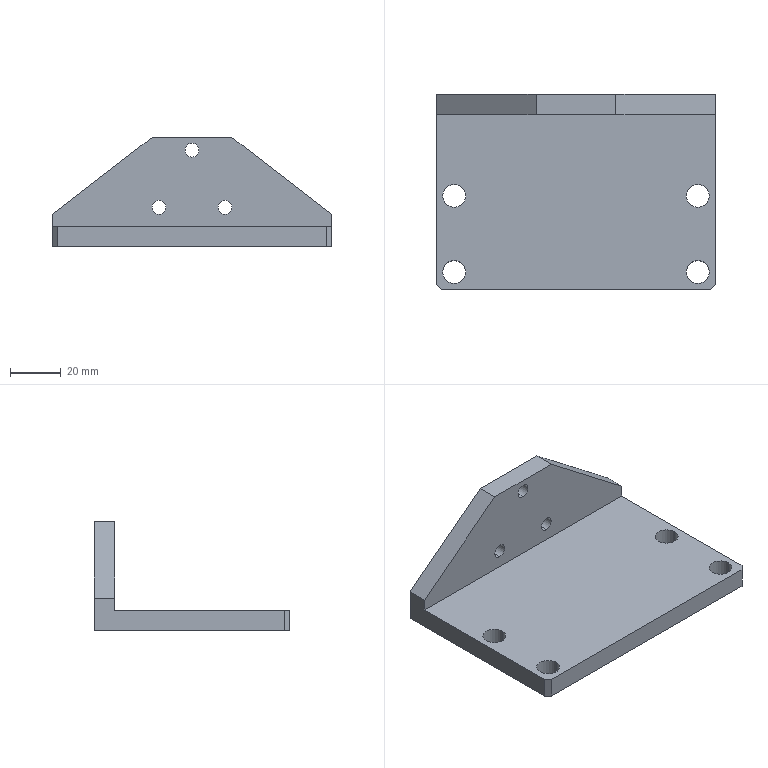Part | SolidWorks | features HoleWzd 2, ICE 2, Chamfer 1, Extrusion 1 | 1 solid | 26 faces | box 110 x 77 x 43 mm | volume 86421 mm3 | cylinder 14 | plane 12 | commonest cylinder face diameters 9 x8 5.5 x6
STEP:
#1=CARTESIAN_POINT('',(-12.99,30.5,12.75));
#2=VERTEX_POINT('',#1);
#3=CARTESIAN_POINT('',(-12.99,30.5,18.25));
#4=VERTEX_POINT('',#3);
#5=CARTESIAN_POINT('',(-12.99,30.5,15.5));
#6=DIRECTION('',(0.,1.,0.));
#7=DIRECTION('',(-1.,0.,0.));
#8=AXIS2_PLACEMENT_3D('',#5,#6,#7);
#9=CIRCLE('',#8,2.75);
#10=EDGE_CURVE('',#2,#4,#9,.T.);
#11=ORIENTED_EDGE('',*,*,#10,.F.);
#12=CARTESIAN_POINT('',(-12.99,38.5,12.75));
#13=VERTEX_POINT('',#12);
#14=CARTESIAN_POINT('',(-12.99,38.5,12.75));
#15=DIRECTION('',(0.,1.,0.));
#16=VECTOR('',#15,1000.);
#17=LINE('',#14,#16);
#18=EDGE_CURVE('',#2,#13,#17,.T.);
#19=ORIENTED_EDGE('',*,*,#18,.T.);
#20=CARTESIAN_POINT('',(-12.99,38.5,18.25));
#21=VERTEX_POINT('',#20);
#22=CARTESIAN_POINT('',(-12.99,38.5,15.5));
#23=DIRECTION('',(0.,1.,0.));
#24=DIRECTION('',(0.,0.,1.));
#25=AXIS2_PLACEMENT_3D('',#22,#23,#24);
#26=CIRCLE('',#25,2.75);
#27=EDGE_CURVE('',#13,#21,#26,.T.);
#28=ORIENTED_EDGE('',*,*,#27,.T.);
#29=CARTESIAN_POINT('',(-12.99,38.5,18.25));
#30=DIRECTION('',(0.,1.,0.));
#31=VECTOR('',#30,1000.);
#32=LINE('',#29,#31);
#33=EDGE_CURVE('',#4,#21,#32,.T.);
#34=ORIENTED_EDGE('',*,*,#33,.F.);
#35=EDGE_LOOP('',(#11,#19,#28,#34));
#36=FACE_OUTER_BOUND('',#35,.T.);
#37=CARTESIAN_POINT('',(-12.99,38.5,15.5));
#38=DIRECTION('',(0.,1.,0.));
#39=DIRECTION('',(0.,0.,1.));
#40=AXIS2_PLACEMENT_3D('',#37,#38,#39);
#41=CYLINDRICAL_SURFACE('',#40,2.75);
#42=ADVANCED_FACE('',(#36),#41,.F.);
#43=CARTESIAN_POINT('',(12.99,30.5,12.75));
#44=VERTEX_POINT('',#43);
#45=CARTESIAN_POINT('',(12.99,30.5,18.25));
#46=VERTEX_POINT('',#45);
#47=CARTESIAN_POINT('',(12.99,30.5,15.5));
#48=DIRECTION('',(0.,1.,0.));
#49=DIRECTION('',(-1.,0.,0.));
#50=AXIS2_PLACEMENT_3D('',#47,#48,#49);
#51=CIRCLE('',#50,2.75);
#52=EDGE_CURVE('',#44,#46,#51,.T.);
#53=ORIENTED_EDGE('',*,*,#52,.F.);
#54=CARTESIAN_POINT('',(12.99,38.5,12.75));
#55=VERTEX_POINT('',#54);
#56=CARTESIAN_POINT('',(12.99,38.5,12.75));
#57=DIRECTION('',(0.,1.,0.));
#58=VECTOR('',#57,1000.);
#59=LINE('',#56,#58);
#60=EDGE_CURVE('',#44,#55,#59,.T.);
#61=ORIENTED_EDGE('',*,*,#60,.T.);
#62=CARTESIAN_POINT('',(12.99,38.5,18.25));
#63=VERTEX_POINT('',#62);
#64=CARTESIAN_POINT('',(12.99,38.5,15.5));
#65=DIRECTION('',(0.,1.,0.));
#66=DIRECTION('',(0.,0.,1.));
#67=AXIS2_PLACEMENT_3D('',#64,#65,#66);
#68=CIRCLE('',#67,2.75);
#69=EDGE_CURVE('',#55,#63,#68,.T.);
#70=ORIENTED_EDGE('',*,*,#69,.T.);
#71=CARTESIAN_POINT('',(12.99,38.5,18.25));
#72=DIRECTION('',(0.,1.,0.));
#73=VECTOR('',#72,1000.);
#74=LINE('',#71,#73);
#75=EDGE_CURVE('',#46,#63,#74,.T.);
#76=ORIENTED_EDGE('',*,*,#75,.F.);
#77=EDGE_LOOP('',(#53,#61,#70,#76));
#78=FACE_OUTER_BOUND('',#77,.T.);
#79=CARTESIAN_POINT('',(12.99,38.5,15.5));
#80=DIRECTION('',(0.,1.,0.));
#81=DIRECTION('',(0.,0.,1.));
#82=AXIS2_PLACEMENT_3D('',#79,#80,#81);
#83=CYLINDRICAL_SURFACE('',#82,2.75);
#84=ADVANCED_FACE('',(#78),#83,.F.);
#85=CARTESIAN_POINT('',(0.,30.5,35.25));
#86=VERTEX_POINT('',#85);
#87=CARTESIAN_POINT('',(0.,30.5,40.75));
#88=VERTEX_POINT('',#87);
#89=CARTESIAN_POINT('',(0.,30.5,38.));
#90=DIRECTION('',(0.,1.,0.));
#91=DIRECTION('',(-1.,0.,0.));
#92=AXIS2_PLACEMENT_3D('',#89,#90,#91);
#93=CIRCLE('',#92,2.75);
#94=EDGE_CURVE('',#86,#88,#93,.T.);
#95=ORIENTED_EDGE('',*,*,#94,.F.);
#96=CARTESIAN_POINT('',(0.,38.5,35.25));
#97=VERTEX_POINT('',#96);
#98=CARTESIAN_POINT('',(0.,38.5,35.25));
#99=DIRECTION('',(0.,1.,0.));
#100=VECTOR('',#99,1000.);
#101=LINE('',#98,#100);
#102=EDGE_CURVE('',#86,#97,#101,.T.);
#103=ORIENTED_EDGE('',*,*,#102,.T.);
#104=CARTESIAN_POINT('',(0.,38.5,40.75));
#105=VERTEX_POINT('',#104);
#106=CARTESIAN_POINT('',(0.,38.5,38.));
#107=DIRECTION('',(0.,1.,0.));
#108=DIRECTION('',(0.,0.,1.));
#109=AXIS2_PLACEMENT_3D('',#106,#107,#108);
#110=CIRCLE('',#109,2.75);
#111=EDGE_CURVE('',#97,#105,#110,.T.);
#112=ORIENTED_EDGE('',*,*,#111,.T.);
#113=CARTESIAN_POINT('',(0.,38.5,40.75));
#114=DIRECTION('',(0.,1.,0.));
#115=VECTOR('',#114,1000.);
#116=LINE('',#113,#115);
#117=EDGE_CURVE('',#88,#105,#116,.T.);
#118=ORIENTED_EDGE('',*,*,#117,.F.);
#119=EDGE_LOOP('',(#95,#103,#112,#118));
#120=FACE_OUTER_BOUND('',#119,.T.);
#121=CARTESIAN_POINT('',(0.,38.5,38.));
#122=DIRECTION('',(0.,1.,0.));
#123=DIRECTION('',(0.,0.,1.));
#124=AXIS2_PLACEMENT_3D('',#121,#122,#123);
#125=CYLINDRICAL_SURFACE('',#124,2.75);
#126=ADVANCED_FACE('',(#120),#125,.F.);
#127=CARTESIAN_POINT('',(-52.5,-31.5,0.));
#128=VERTEX_POINT('',#127);
#129=CARTESIAN_POINT('',(-43.5,-31.5,0.));
#130=VERTEX_POINT('',#129);
#131=CARTESIAN_POINT('',(-48.,-31.5,0.));
#132=DIRECTION('',(0.,0.,1.));
#133=DIRECTION('',(1.,0.,0.));
#134=AXIS2_PLACEMENT_3D('',#131,#132,#133);
#135=CIRCLE('',#134,4.5);
#136=EDGE_CURVE('',#128,#130,#135,.T.);
#137=ORIENTED_EDGE('',*,*,#136,.F.);
#138=CARTESIAN_POINT('',(-52.5,-31.5,8.));
#139=VERTEX_POINT('',#138);
#140=CARTESIAN_POINT('',(-52.5,-31.5,8.));
#141=DIRECTION('',(0.,0.,1.));
#142=VECTOR('',#141,1000.);
#143=LINE('',#140,#142);
#144=EDGE_CURVE('',#128,#139,#143,.T.);
#145=ORIENTED_EDGE('',*,*,#144,.T.);
#146=CARTESIAN_POINT('',(-43.5,-31.5,8.));
#147=VERTEX_POINT('',#146);
#148=CARTESIAN_POINT('',(-48.,-31.5,8.));
#149=DIRECTION('',(0.,0.,1.));
#150=DIRECTION('',(1.,0.,0.));
#151=AXIS2_PLACEMENT_3D('',#148,#149,#150);
#152=CIRCLE('',#151,4.5);
#153=EDGE_CURVE('',#139,#147,#152,.T.);
#154=ORIENTED_EDGE('',*,*,#153,.T.);
#155=CARTESIAN_POINT('',(-43.5,-31.5,8.));
#156=DIRECTION('',(0.,0.,1.));
#157=VECTOR('',#156,1000.);
#158=LINE('',#155,#157);
#159=EDGE_CURVE('',#130,#147,#158,.T.);
#160=ORIENTED_EDGE('',*,*,#159,.F.);
#161=EDGE_LOOP('',(#137,#145,#154,#160));
#162=FACE_OUTER_BOUND('',#161,.T.);
#163=CARTESIAN_POINT('',(-48.,-31.5,8.));
#164=DIRECTION('',(0.,0.,1.));
#165=DIRECTION('',(1.,0.,0.));
#166=AXIS2_PLACEMENT_3D('',#163,#164,#165);
#167=CYLINDRICAL_SURFACE('',#166,4.5);
#168=ADVANCED_FACE('',(#162),#167,.F.);
#169=CARTESIAN_POINT('',(43.5,-31.5,0.));
#170=VERTEX_POINT('',#169);
#171=CARTESIAN_POINT('',(52.5,-31.5,0.));
#172=VERTEX_POINT('',#171);
#173=CARTESIAN_POINT('',(48.,-31.5,0.));
#174=DIRECTION('',(0.,0.,1.));
#175=DIRECTION('',(1.,0.,0.));
#176=AXIS2_PLACEMENT_3D('',#173,#174,#175);
#177=CIRCLE('',#176,4.5);
#178=EDGE_CURVE('',#170,#172,#177,.T.);
#179=ORIENTED_EDGE('',*,*,#178,.F.);
#180=CARTESIAN_POINT('',(43.5,-31.5,8.));
#181=VERTEX_POINT('',#180);
#182=CARTESIAN_POINT('',(43.5,-31.5,8.));
#183=DIRECTION('',(0.,0.,1.));
#184=VECTOR('',#183,1000.);
#185=LINE('',#182,#184);
#186=EDGE_CURVE('',#170,#181,#185,.T.);
#187=ORIENTED_EDGE('',*,*,#186,.T.);
#188=CARTESIAN_POINT('',(52.5,-31.5,8.));
#189=VERTEX_POINT('',#188);
#190=CARTESIAN_POINT('',(48.,-31.5,8.));
#191=DIRECTION('',(0.,0.,1.));
#192=DIRECTION('',(1.,0.,0.));
#193=AXIS2_PLACEMENT_3D('',#190,#191,#192);
#194=CIRCLE('',#193,4.5);
#195=EDGE_CURVE('',#181,#189,#194,.T.);
#196=ORIENTED_EDGE('',*,*,#195,.T.);
#197=CARTESIAN_POINT('',(52.5,-31.5,8.));
#198=DIRECTION('',(0.,0.,1.));
#199=VECTOR('',#198,1000.);
#200=LINE('',#197,#199);
#201=EDGE_CURVE('',#172,#189,#200,.T.);
#202=ORIENTED_EDGE('',*,*,#201,.F.);
#203=EDGE_LOOP('',(#179,#187,#196,#202));
#204=FACE_OUTER_BOUND('',#203,.T.);
#205=CARTESIAN_POINT('',(48.,-31.5,8.));
#206=DIRECTION('',(0.,0.,1.));
#207=DIRECTION('',(1.,0.,0.));
#208=AXIS2_PLACEMENT_3D('',#205,#206,#207);
#209=CYLINDRICAL_SURFACE('',#208,4.5);
#210=ADVANCED_FACE('',(#204),#209,.F.);
#211=CARTESIAN_POINT('',(43.5,-1.5,0.));
#212=VERTEX_POINT('',#211);
#213=CARTESIAN_POINT('',(52.5,-1.5,0.));
#214=VERTEX_POINT('',#213);
#215=CARTESIAN_POINT('',(48.,-1.5,0.));
#216=DIRECTION('',(0.,0.,1.));
#217=DIRECTION('',(1.,0.,0.));
#218=AXIS2_PLACEMENT_3D('',#215,#216,#217);
#219=CIRCLE('',#218,4.5);
#220=EDGE_CURVE('',#212,#214,#219,.T.);
#221=ORIENTED_EDGE('',*,*,#220,.F.);
#222=CARTESIAN_POINT('',(43.5,-1.5,8.));
#223=VERTEX_POINT('',#222);
#224=CARTESIAN_POINT('',(43.5,-1.5,8.));
#225=DIRECTION('',(0.,0.,1.));
#226=VECTOR('',#225,1000.);
#227=LINE('',#224,#226);
#228=EDGE_CURVE('',#212,#223,#227,.T.);
#229=ORIENTED_EDGE('',*,*,#228,.T.);
#230=CARTESIAN_POINT('',(52.5,-1.5,8.));
#231=VERTEX_POINT('',#230);
#232=CARTESIAN_POINT('',(48.,-1.5,8.));
#233=DIRECTION('',(0.,0.,1.));
#234=DIRECTION('',(1.,0.,0.));
#235=AXIS2_PLACEMENT_3D('',#232,#233,#234);
#236=CIRCLE('',#235,4.5);
#237=EDGE_CURVE('',#223,#231,#236,.T.);
#238=ORIENTED_EDGE('',*,*,#237,.T.);
#239=CARTESIAN_POINT('',(52.5,-1.5,8.));
#240=DIRECTION('',(0.,0.,1.));
#241=VECTOR('',#240,1000.);
#242=LINE('',#239,#241);
#243=EDGE_CURVE('',#214,#231,#242,.T.);
#244=ORIENTED_EDGE('',*,*,#243,.F.);
#245=EDGE_LOOP('',(#221,#229,#238,#244));
#246=FACE_OUTER_BOUND('',#245,.T.);
#247=CARTESIAN_POINT('',(48.,-1.5,8.));
#248=DIRECTION('',(0.,0.,1.));
#249=DIRECTION('',(1.,0.,0.));
#250=AXIS2_PLACEMENT_3D('',#247,#248,#249);
#251=CYLINDRICAL_SURFACE('',#250,4.5);
#252=ADVANCED_FACE('',(#246),#251,.F.);
#253=CARTESIAN_POINT('',(-52.5,-1.5,0.));
#254=VERTEX_POINT('',#253);
#255=CARTESIAN_POINT('',(-43.5,-1.5,0.));
#256=VERTEX_POINT('',#255);
#257=CARTESIAN_POINT('',(-48.,-1.5,0.));
#258=DIRECTION('',(0.,0.,1.));
#259=DIRECTION('',(1.,0.,0.));
#260=AXIS2_PLACEMENT_3D('',#257,#258,#259);
#261=CIRCLE('',#260,4.5);
#262=EDGE_CURVE('',#254,#256,#261,.T.);
#263=ORIENTED_EDGE('',*,*,#262,.F.);
#264=CARTESIAN_POINT('',(-52.5,-1.5,8.));
#265=VERTEX_POINT('',#264);
#266=CARTESIAN_POINT('',(-52.5,-1.5,8.));
#267=DIRECTION('',(0.,0.,1.));
#268=VECTOR('',#267,1000.);
#269=LINE('',#266,#268);
#270=EDGE_CURVE('',#254,#265,#269,.T.);
#271=ORIENTED_EDGE('',*,*,#270,.T.);
#272=CARTESIAN_POINT('',(-43.5,-1.5,8.));
#273=VERTEX_POINT('',#272);
#274=CARTESIAN_POINT('',(-48.,-1.5,8.));
#275=DIRECTION('',(0.,0.,1.));
#276=DIRECTION('',(1.,0.,0.));
#277=AXIS2_PLACEMENT_3D('',#274,#275,#276);
#278=CIRCLE('',#277,4.5);
#279=EDGE_CURVE('',#265,#273,#278,.T.);
#280=ORIENTED_EDGE('',*,*,#279,.T.);
#281=CARTESIAN_POINT('',(-43.5,-1.5,8.));
#282=DIRECTION('',(0.,0.,1.));
#283=VECTOR('',#282,1000.);
#284=LINE('',#281,#283);
#285=EDGE_CURVE('',#256,#273,#284,.T.);
#286=ORIENTED_EDGE('',*,*,#285,.F.);
#287=EDGE_LOOP('',(#263,#271,#280,#286));
#288=FACE_OUTER_BOUND('',#287,.T.);
#289=CARTESIAN_POINT('',(-48.,-1.5,8.));
#290=DIRECTION('',(0.,0.,1.));
#291=DIRECTION('',(1.,0.,0.));
#292=AXIS2_PLACEMENT_3D('',#289,#290,#291);
#293=CYLINDRICAL_SURFACE('',#292,4.5);
#294=ADVANCED_FACE('',(#288),#293,.F.);
#295=CARTESIAN_POINT('',(55.,-36.5,8.));
#296=VERTEX_POINT('',#295);
#297=CARTESIAN_POINT('',(55.,30.5,8.));
#298=VERTEX_POINT('',#297);
#299=CARTESIAN_POINT('',(55.,38.5,8.));
#300=DIRECTION('',(0.,1.,0.));
#301=VECTOR('',#300,1000.);
#302=LINE('',#299,#301);
#303=EDGE_CURVE('',#296,#298,#302,.T.);
#304=ORIENTED_EDGE('',*,*,#303,.F.);
#305=CARTESIAN_POINT('',(55.,-36.5,0.));
#306=VERTEX_POINT('',#305);
#307=CARTESIAN_POINT('',(55.,-36.5,8.));
#308=DIRECTION('',(0.,0.,-1.));
#309=VECTOR('',#308,1000.);
#310=LINE('',#307,#309);
#311=EDGE_CURVE('',#296,#306,#310,.T.);
#312=ORIENTED_EDGE('',*,*,#311,.T.);
#313=CARTESIAN_POINT('',(55.,38.5,0.));
#314=VERTEX_POINT('',#313);
#315=CARTESIAN_POINT('',(55.,38.5,0.));
#316=DIRECTION('',(0.,1.,0.));
#317=VECTOR('',#316,1000.);
#318=LINE('',#315,#317);
#319=EDGE_CURVE('',#306,#314,#318,.T.);
#320=ORIENTED_EDGE('',*,*,#319,.T.);
#321=CARTESIAN_POINT('',(55.,38.5,12.75));
#322=VERTEX_POINT('',#321);
#323=CARTESIAN_POINT('',(55.,38.5,8.));
#324=DIRECTION('',(0.,0.,-1.));
#325=VECTOR('',#324,1000.);
#326=LINE('',#323,#325);
#327=EDGE_CURVE('',#322,#314,#326,.T.);
#328=ORIENTED_EDGE('',*,*,#327,.F.);
#329=CARTESIAN_POINT('',(55.,30.5,12.75));
#330=VERTEX_POINT('',#329);
#331=CARTESIAN_POINT('',(55.,-4.5,12.75));
#332=DIRECTION('',(0.,1.,0.));
#333=VECTOR('',#332,1000.);
#334=LINE('',#331,#333);
#335=EDGE_CURVE('',#330,#322,#334,.T.);
#336=ORIENTED_EDGE('',*,*,#335,.F.);
#337=CARTESIAN_POINT('',(55.,30.5,43.));
#338=DIRECTION('',(0.,0.,-1.));
#339=VECTOR('',#338,1000.);
#340=LINE('',#337,#339);
#341=EDGE_CURVE('',#330,#298,#340,.T.);
#342=ORIENTED_EDGE('',*,*,#341,.T.);
#343=EDGE_LOOP('',(#304,#312,#320,#328,#336,#342));
#344=FACE_OUTER_BOUND('',#343,.T.);
#345=CARTESIAN_POINT('',(55.,38.5,8.));
#346=DIRECTION('',(-1.,0.,0.));
#347=DIRECTION('',(0.,-1.,0.));
#348=AXIS2_PLACEMENT_3D('',#345,#346,#347);
#349=PLANE('',#348);
#350=ADVANCED_FACE('',(#344),#349,.F.);
#351=CARTESIAN_POINT('',(-12.99,38.5,15.5));
#352=DIRECTION('',(0.,1.,0.));
#353=DIRECTION('',(0.,0.,1.));
#354=AXIS2_PLACEMENT_3D('',#351,#352,#353);
#355=CIRCLE('',#354,2.75);
#356=EDGE_CURVE('',#21,#13,#355,.T.);
#357=ORIENTED_EDGE('',*,*,#356,.F.);
#358=ORIENTED_EDGE('',*,*,#27,.F.);
#359=EDGE_LOOP('',(#357,#358));
#360=FACE_BOUND('',#359,.T.);
#361=CARTESIAN_POINT('',(12.99,38.5,15.5));
#362=DIRECTION('',(0.,1.,0.));
#363=DIRECTION('',(0.,0.,1.));
#364=AXIS2_PLACEMENT_3D('',#361,#362,#363);
#365=CIRCLE('',#364,2.75);
#366=EDGE_CURVE('',#63,#55,#365,.T.);
#367=ORIENTED_EDGE('',*,*,#366,.F.);
#368=ORIENTED_EDGE('',*,*,#69,.F.);
#369=EDGE_LOOP('',(#367,#368));
#370=FACE_BOUND('',#369,.T.);
#371=CARTESIAN_POINT('',(0.,38.5,38.));
#372=DIRECTION('',(0.,1.,0.));
#373=DIRECTION('',(0.,0.,1.));
#374=AXIS2_PLACEMENT_3D('',#371,#372,#373);
#375=CIRCLE('',#374,2.75);
#376=EDGE_CURVE('',#105,#97,#375,.T.);
#377=ORIENTED_EDGE('',*,*,#376,.F.);
#378=ORIENTED_EDGE('',*,*,#111,.F.);
#379=EDGE_LOOP('',(#377,#378));
#380=FACE_BOUND('',#379,.T.);
#381=CARTESIAN_POINT('',(15.74,38.5,43.));
#382=VERTEX_POINT('',#381);
#383=CARTESIAN_POINT('',(15.74,38.5,43.));
#384=DIRECTION('',(0.7921,0.,-0.6103));
#385=VECTOR('',#384,1000.);
#386=LINE('',#383,#385);
#387=EDGE_CURVE('',#382,#322,#386,.T.);
#388=ORIENTED_EDGE('',*,*,#387,.T.);
#389=ORIENTED_EDGE('',*,*,#327,.T.);
#390=CARTESIAN_POINT('',(-55.,38.5,0.));
#391=VERTEX_POINT('',#390);
#392=CARTESIAN_POINT('',(-55.,38.5,0.));
#393=DIRECTION('',(-1.,0.,0.));
#394=VECTOR('',#393,1000.);
#395=LINE('',#392,#394);
#396=EDGE_CURVE('',#314,#391,#395,.T.);
#397=ORIENTED_EDGE('',*,*,#396,.T.);
#398=CARTESIAN_POINT('',(-55.,38.5,12.75));
#399=VERTEX_POINT('',#398);
#400=CARTESIAN_POINT('',(-55.,38.5,8.));
#401=DIRECTION('',(0.,0.,-1.));
#402=VECTOR('',#401,1000.);
#403=LINE('',#400,#402);
#404=EDGE_CURVE('',#399,#391,#403,.T.);
#405=ORIENTED_EDGE('',*,*,#404,.F.);
#406=CARTESIAN_POINT('',(-15.74,38.5,43.));
#407=VERTEX_POINT('',#406);
#408=CARTESIAN_POINT('',(-55.,38.5,12.75));
#409=DIRECTION('',(0.7921,0.,0.6103));
#410=VECTOR('',#409,1000.);
#411=LINE('',#408,#410);
#412=EDGE_CURVE('',#399,#407,#411,.T.);
#413=ORIENTED_EDGE('',*,*,#412,.T.);
#414=CARTESIAN_POINT('',(-55.,38.5,43.));
#415=DIRECTION('',(1.,0.,0.));
#416=VECTOR('',#415,1000.);
#417=LINE('',#414,#416);
#418=EDGE_CURVE('',#407,#382,#417,.T.);
#419=ORIENTED_EDGE('',*,*,#418,.T.);
#420=EDGE_LOOP('',(#388,#389,#397,#405,#413,#419));
#421=FACE_OUTER_BOUND('',#420,.T.);
#422=CARTESIAN_POINT('',(-55.,38.5,8.));
#423=DIRECTION('',(0.,-1.,0.));
#424=DIRECTION('',(0.,0.,-1.));
#425=AXIS2_PLACEMENT_3D('',#422,#423,#424);
#426=PLANE('',#425);
#427=ADVANCED_FACE('',(#360,#370,#380,#421),#426,.F.);
#428=CARTESIAN_POINT('',(-55.,-36.5,0.));
#429=VERTEX_POINT('',#428);
#430=CARTESIAN_POINT('',(-55.,38.5,0.));
#431=DIRECTION('',(0.,-1.,0.));
#432=VECTOR('',#431,1000.);
#433=LINE('',#430,#432);
#434=EDGE_CURVE('',#391,#429,#433,.T.);
#435=ORIENTED_EDGE('',*,*,#434,.T.);
#436=CARTESIAN_POINT('',(-55.,-36.5,8.));
#437=VERTEX_POINT('',#436);
#438=CARTESIAN_POINT('',(-55.,-36.5,8.));
#439=DIRECTION('',(0.,0.,1.));
#440=VECTOR('',#439,1000.);
#441=LINE('',#438,#440);
#442=EDGE_CURVE('',#429,#437,#441,.T.);
#443=ORIENTED_EDGE('',*,*,#442,.T.);
#444=CARTESIAN_POINT('',(-55.,30.5,8.));
#445=VERTEX_POINT('',#444);
#446=CARTESIAN_POINT('',(-55.,38.5,8.));
#447=DIRECTION('',(0.,-1.,0.));
#448=VECTOR('',#447,1000.);
#449=LINE('',#446,#448);
#450=EDGE_CURVE('',#445,#437,#449,.T.);
#451=ORIENTED_EDGE('',*,*,#450,.F.);
#452=CARTESIAN_POINT('',(-55.,30.5,12.75));
#453=VERTEX_POINT('',#452);
#454=CARTESIAN_POINT('',(-55.,30.5,43.));
#455=DIRECTION('',(0.,0.,-1.));
#456=VECTOR('',#455,1000.);
#457=LINE('',#454,#456);
#458=EDGE_CURVE('',#453,#445,#457,.T.);
#459=ORIENTED_EDGE('',*,*,#458,.F.);
#460=CARTESIAN_POINT('',(-55.,-4.5,12.75));
#461=DIRECTION('',(0.,1.,0.));
#462=VECTOR('',#461,1000.);
#463=LINE('',#460,#462);
#464=EDGE_CURVE('',#453,#399,#463,.T.);
#465=ORIENTED_EDGE('',*,*,#464,.T.);
#466=ORIENTED_EDGE('',*,*,#404,.T.);
#467=EDGE_LOOP('',(#435,#443,#451,#459,#465,#466));
#468=FACE_OUTER_BOUND('',#467,.T.);
#469=CARTESIAN_POINT('',(-55.,38.5,8.));
#470=DIRECTION('',(1.,0.,0.));
#471=DIRECTION('',(0.,1.,0.));
#472=AXIS2_PLACEMENT_3D('',#469,#470,#471);
#473=PLANE('',#472);
#474=ADVANCED_FACE('',(#468),#473,.F.);
#475=CARTESIAN_POINT('',(-12.99,30.5,15.5));
#476=DIRECTION('',(0.,1.,0.));
#477=DIRECTION('',(-1.,0.,0.));
#478=AXIS2_PLACEMENT_3D('',#475,#476,#477);
#479=CIRCLE('',#478,2.75);
#480=EDGE_CURVE('',#4,#2,#479,.T.);
#481=ORIENTED_EDGE('',*,*,#480,.T.);
#482=ORIENTED_EDGE('',*,*,#10,.T.);
#483=EDGE_LOOP('',(#481,#482));
#484=FACE_BOUND('',#483,.T.);
#485=CARTESIAN_POINT('',(12.99,30.5,15.5));
#486=DIRECTION('',(0.,1.,0.));
#487=DIRECTION('',(-1.,0.,0.));
#488=AXIS2_PLACEMENT_3D('',#485,#486,#487);
#489=CIRCLE('',#488,2.75);
#490=EDGE_CURVE('',#46,#44,#489,.T.);
#491=ORIENTED_EDGE('',*,*,#490,.T.);
#492=ORIENTED_EDGE('',*,*,#52,.T.);
#493=EDGE_LOOP('',(#491,#492));
#494=FACE_BOUND('',#493,.T.);
#495=CARTESIAN_POINT('',(0.,30.5,38.));
#496=DIRECTION('',(0.,1.,0.));
#497=DIRECTION('',(-1.,0.,0.));
#498=AXIS2_PLACEMENT_3D('',#495,#496,#497);
#499=CIRCLE('',#498,2.75);
#500=EDGE_CURVE('',#88,#86,#499,.T.);
#501=ORIENTED_EDGE('',*,*,#500,.T.);
#502=ORIENTED_EDGE('',*,*,#94,.T.);
#503=EDGE_LOOP('',(#501,#502));
#504=FACE_BOUND('',#503,.T.);
#505=CARTESIAN_POINT('',(15.74,30.5,43.));
#506=VERTEX_POINT('',#505);
#507=CARTESIAN_POINT('',(-28.648,30.5,77.201));
#508=DIRECTION('',(0.7921,0.,-0.6103));
#509=VECTOR('',#508,1000.);
#510=LINE('',#507,#509);
#511=EDGE_CURVE('',#506,#330,#510,.T.);
#512=ORIENTED_EDGE('',*,*,#511,.F.);
#513=CARTESIAN_POINT('',(-15.74,30.5,43.));
#514=VERTEX_POINT('',#513);
#515=CARTESIAN_POINT('',(-55.,30.5,43.));
#516=DIRECTION('',(1.,0.,0.));
#517=VECTOR('',#516,1000.);
#518=LINE('',#515,#517);
#519=EDGE_CURVE('',#514,#506,#518,.T.);
#520=ORIENTED_EDGE('',*,*,#519,.F.);
#521=CARTESIAN_POINT('',(-40.375,30.5,24.019));
#522=DIRECTION('',(0.7921,0.,0.6103));
#523=VECTOR('',#522,1000.);
#524=LINE('',#521,#523);
#525=EDGE_CURVE('',#453,#514,#524,.T.);
#526=ORIENTED_EDGE('',*,*,#525,.F.);
#527=ORIENTED_EDGE('',*,*,#458,.T.);
#528=CARTESIAN_POINT('',(0.,30.5,8.));
#529=DIRECTION('',(-1.,0.,0.));
#530=VECTOR('',#529,1000.);
#531=LINE('',#528,#530);
#532=EDGE_CURVE('',#298,#445,#531,.T.);
#533=ORIENTED_EDGE('',*,*,#532,.F.);
#534=ORIENTED_EDGE('',*,*,#341,.F.);
#535=EDGE_LOOP('',(#512,#520,#526,#527,#533,#534));
#536=FACE_OUTER_BOUND('',#535,.T.);
#537=CARTESIAN_POINT('',(-55.,30.5,43.));
#538=DIRECTION('',(0.,1.,0.));
#539=DIRECTION('',(-1.,0.,0.));
#540=AXIS2_PLACEMENT_3D('',#537,#538,#539);
#541=PLANE('',#540);
#542=ADVANCED_FACE('',(#484,#494,#504,#536),#541,.F.);
#543=ORIENTED_EDGE('',*,*,#519,.T.);
#544=CARTESIAN_POINT('',(15.74,0.,43.));
#545=DIRECTION('',(0.,1.,0.));
#546=VECTOR('',#545,1000.);
#547=LINE('',#544,#546);
#548=EDGE_CURVE('',#506,#382,#547,.T.);
#549=ORIENTED_EDGE('',*,*,#548,.T.);
#550=ORIENTED_EDGE('',*,*,#418,.F.);
#551=CARTESIAN_POINT('',(-15.74,0.,43.));
#552=DIRECTION('',(0.,-1.,0.));
#553=VECTOR('',#552,1000.);
#554=LINE('',#551,#553);
#555=EDGE_CURVE('',#407,#514,#554,.T.);
#556=ORIENTED_EDGE('',*,*,#555,.T.);
#557=EDGE_LOOP('',(#543,#549,#550,#556));
#558=FACE_OUTER_BOUND('',#557,.T.);
#559=CARTESIAN_POINT('',(0.,0.,43.));
#560=DIRECTION('',(0.,0.,1.));
#561=DIRECTION('',(1.,0.,0.));
#562=AXIS2_PLACEMENT_3D('',#559,#560,#561);
#563=PLANE('',#562);
#564=ADVANCED_FACE('',(#558),#563,.T.);
#565=CARTESIAN_POINT('',(-48.,-31.5,8.));
#566=DIRECTION('',(0.,0.,1.));
#567=DIRECTION('',(1.,0.,0.));
#568=AXIS2_PLACEMENT_3D('',#565,#566,#567);
#569=CIRCLE('',#568,4.5);
#570=EDGE_CURVE('',#147,#139,#569,.T.);
#571=ORIENTED_EDGE('',*,*,#570,.F.);
#572=ORIENTED_EDGE('',*,*,#153,.F.);
#573=EDGE_LOOP('',(#571,#572));
#574=FACE_BOUND('',#573,.T.);
#575=CARTESIAN_POINT('',(48.,-31.5,8.));
#576=DIRECTION('',(0.,0.,1.));
#577=DIRECTION('',(1.,0.,0.));
#578=AXIS2_PLACEMENT_3D('',#575,#576,#577);
#579=CIRCLE('',#578,4.5);
#580=EDGE_CURVE('',#189,#181,#579,.T.);
#581=ORIENTED_EDGE('',*,*,#580,.F.);
#582=ORIENTED_EDGE('',*,*,#195,.F.);
#583=EDGE_LOOP('',(#581,#582));
#584=FACE_BOUND('',#583,.T.);
#585=CARTESIAN_POINT('',(48.,-1.5,8.));
#586=DIRECTION('',(0.,0.,1.));
#587=DIRECTION('',(1.,0.,0.));
#588=AXIS2_PLACEMENT_3D('',#585,#586,#587);
#589=CIRCLE('',#588,4.5);
#590=EDGE_CURVE('',#231,#223,#589,.T.);
#591=ORIENTED_EDGE('',*,*,#590,.F.);
#592=ORIENTED_EDGE('',*,*,#237,.F.);
#593=EDGE_LOOP('',(#591,#592));
#594=FACE_BOUND('',#593,.T.);
#595=CARTESIAN_POINT('',(-48.,-1.5,8.));
#596=DIRECTION('',(0.,0.,1.));
#597=DIRECTION('',(1.,0.,0.));
#598=AXIS2_PLACEMENT_3D('',#595,#596,#597);
#599=CIRCLE('',#598,4.5);
#600=EDGE_CURVE('',#273,#265,#599,.T.);
#601=ORIENTED_EDGE('',*,*,#600,.F.);
#602=ORIENTED_EDGE('',*,*,#279,.F.);
#603=EDGE_LOOP('',(#601,#602));
#604=FACE_BOUND('',#603,.T.);
#605=ORIENTED_EDGE('',*,*,#450,.T.);
#606=CARTESIAN_POINT('',(-53.,-38.5,8.));
#607=VERTEX_POINT('',#606);
#608=CARTESIAN_POINT('',(-45.75,-45.75,8.));
#609=DIRECTION('',(0.7071,-0.7071,0.));
#610=VECTOR('',#609,1000.);
#611=LINE('',#608,#610);
#612=EDGE_CURVE('',#437,#607,#611,.T.);
#613=ORIENTED_EDGE('',*,*,#612,.T.);
#614=CARTESIAN_POINT('',(53.,-38.5,8.));
#615=VERTEX_POINT('',#614);
#616=CARTESIAN_POINT('',(-55.,-38.5,8.));
#617=DIRECTION('',(1.,0.,0.));
#618=VECTOR('',#617,1000.);
#619=LINE('',#616,#618);
#620=EDGE_CURVE('',#607,#615,#619,.T.);
#621=ORIENTED_EDGE('',*,*,#620,.T.);
#622=CARTESIAN_POINT('',(45.75,-45.75,8.));
#623=DIRECTION('',(0.7071,0.7071,0.));
#624=VECTOR('',#623,1000.);
#625=LINE('',#622,#624);
#626=EDGE_CURVE('',#615,#296,#625,.T.);
#627=ORIENTED_EDGE('',*,*,#626,.T.);
#628=ORIENTED_EDGE('',*,*,#303,.T.);
#629=ORIENTED_EDGE('',*,*,#532,.T.);
#630=EDGE_LOOP('',(#605,#613,#621,#627,#628,#629));
#631=FACE_OUTER_BOUND('',#630,.T.);
#632=CARTESIAN_POINT('',(0.,0.,8.));
#633=DIRECTION('',(0.,0.,1.));
#634=DIRECTION('',(1.,0.,0.));
#635=AXIS2_PLACEMENT_3D('',#632,#633,#634);
#636=PLANE('',#635);
#637=ADVANCED_FACE('',(#574,#584,#594,#604,#631),#636,.T.);
#638=ORIENTED_EDGE('',*,*,#620,.F.);
#639=CARTESIAN_POINT('',(-53.,-38.5,0.));
#640=VERTEX_POINT('',#639);
#641=CARTESIAN_POINT('',(-53.,-38.5,8.));
#642=DIRECTION('',(0.,0.,-1.));
#643=VECTOR('',#642,1000.);
#644=LINE('',#641,#643);
#645=EDGE_CURVE('',#607,#640,#644,.T.);
#646=ORIENTED_EDGE('',*,*,#645,.T.);
#647=CARTESIAN_POINT('',(53.,-38.5,0.));
#648=VERTEX_POINT('',#647);
#649=CARTESIAN_POINT('',(-55.,-38.5,0.));
#650=DIRECTION('',(1.,0.,0.));
#651=VECTOR('',#650,1000.);
#652=LINE('',#649,#651);
#653=EDGE_CURVE('',#640,#648,#652,.T.);
#654=ORIENTED_EDGE('',*,*,#653,.T.);
#655=CARTESIAN_POINT('',(53.,-38.5,8.));
#656=DIRECTION('',(0.,0.,1.));
#657=VECTOR('',#656,1000.);
#658=LINE('',#655,#657);
#659=EDGE_CURVE('',#648,#615,#658,.T.);
#660=ORIENTED_EDGE('',*,*,#659,.T.);
#661=EDGE_LOOP('',(#638,#646,#654,#660));
#662=FACE_OUTER_BOUND('',#661,.T.);
#663=CARTESIAN_POINT('',(-55.,-38.5,8.));
#664=DIRECTION('',(0.,1.,0.));
#665=DIRECTION('',(0.,0.,1.));
#666=AXIS2_PLACEMENT_3D('',#663,#664,#665);
#667=PLANE('',#666);
#668=ADVANCED_FACE('',(#662),#667,.F.);
#669=CARTESIAN_POINT('',(-48.,-31.5,0.));
#670=DIRECTION('',(0.,0.,1.));
#671=DIRECTION('',(1.,0.,0.));
#672=AXIS2_PLACEMENT_3D('',#669,#670,#671);
#673=CIRCLE('',#672,4.5);
#674=EDGE_CURVE('',#130,#128,#673,.T.);
#675=ORIENTED_EDGE('',*,*,#674,.T.);
#676=ORIENTED_EDGE('',*,*,#136,.T.);
#677=EDGE_LOOP('',(#675,#676));
#678=FACE_BOUND('',#677,.T.);
#679=CARTESIAN_POINT('',(48.,-31.5,0.));
#680=DIRECTION('',(0.,0.,1.));
#681=DIRECTION('',(1.,0.,0.));
#682=AXIS2_PLACEMENT_3D('',#679,#680,#681);
#683=CIRCLE('',#682,4.5);
#684=EDGE_CURVE('',#172,#170,#683,.T.);
#685=ORIENTED_EDGE('',*,*,#684,.T.);
#686=ORIENTED_EDGE('',*,*,#178,.T.);
#687=EDGE_LOOP('',(#685,#686));
#688=FACE_BOUND('',#687,.T.);
#689=CARTESIAN_POINT('',(48.,-1.5,0.));
#690=DIRECTION('',(0.,0.,1.));
#691=DIRECTION('',(1.,0.,0.));
#692=AXIS2_PLACEMENT_3D('',#689,#690,#691);
#693=CIRCLE('',#692,4.5);
#694=EDGE_CURVE('',#214,#212,#693,.T.);
#695=ORIENTED_EDGE('',*,*,#694,.T.);
#696=ORIENTED_EDGE('',*,*,#220,.T.);
#697=EDGE_LOOP('',(#695,#696));
#698=FACE_BOUND('',#697,.T.);
#699=CARTESIAN_POINT('',(-48.,-1.5,0.));
#700=DIRECTION('',(0.,0.,1.));
#701=DIRECTION('',(1.,0.,0.));
#702=AXIS2_PLACEMENT_3D('',#699,#700,#701);
#703=CIRCLE('',#702,4.5);
#704=EDGE_CURVE('',#256,#254,#703,.T.);
#705=ORIENTED_EDGE('',*,*,#704,.T.);
#706=ORIENTED_EDGE('',*,*,#262,.T.);
#707=EDGE_LOOP('',(#705,#706));
#708=FACE_BOUND('',#707,.T.);
#709=ORIENTED_EDGE('',*,*,#653,.F.);
#710=CARTESIAN_POINT('',(-53.,-38.5,0.));
#711=DIRECTION('',(-0.7071,0.7071,0.));
#712=VECTOR('',#711,1000.);
#713=LINE('',#710,#712);
#714=EDGE_CURVE('',#640,#429,#713,.T.);
#715=ORIENTED_EDGE('',*,*,#714,.T.);
#716=ORIENTED_EDGE('',*,*,#434,.F.);
#717=ORIENTED_EDGE('',*,*,#396,.F.);
#718=ORIENTED_EDGE('',*,*,#319,.F.);
#719=CARTESIAN_POINT('',(55.,-36.5,0.));
#720=DIRECTION('',(-0.7071,-0.7071,0.));
#721=VECTOR('',#720,1000.);
#722=LINE('',#719,#721);
#723=EDGE_CURVE('',#306,#648,#722,.T.);
#724=ORIENTED_EDGE('',*,*,#723,.T.);
#725=EDGE_LOOP('',(#709,#715,#716,#717,#718,#724));
#726=FACE_OUTER_BOUND('',#725,.T.);
#727=CARTESIAN_POINT('',(0.,0.,0.));
#728=DIRECTION('',(0.,0.,1.));
#729=DIRECTION('',(1.,0.,0.));
#730=AXIS2_PLACEMENT_3D('',#727,#728,#729);
#731=PLANE('',#730);
#732=ADVANCED_FACE('',(#678,#688,#698,#708,#726),#731,.F.);
#733=ORIENTED_EDGE('',*,*,#525,.T.);
#734=ORIENTED_EDGE('',*,*,#555,.F.);
#735=ORIENTED_EDGE('',*,*,#412,.F.);
#736=ORIENTED_EDGE('',*,*,#464,.F.);
#737=EDGE_LOOP('',(#733,#734,#735,#736));
#738=FACE_OUTER_BOUND('',#737,.T.);
#739=CARTESIAN_POINT('',(-55.,-4.5,12.75));
#740=DIRECTION('',(-0.6103,0.,0.7921));
#741=DIRECTION('',(0.7921,0.,0.6103));
#742=AXIS2_PLACEMENT_3D('',#739,#740,#741);
#743=PLANE('',#742);
#744=ADVANCED_FACE('',(#738),#743,.T.);
#745=ORIENTED_EDGE('',*,*,#511,.T.);
#746=ORIENTED_EDGE('',*,*,#335,.T.);
#747=ORIENTED_EDGE('',*,*,#387,.F.);
#748=ORIENTED_EDGE('',*,*,#548,.F.);
#749=EDGE_LOOP('',(#745,#746,#747,#748));
#750=FACE_OUTER_BOUND('',#749,.T.);
#751=CARTESIAN_POINT('',(15.74,-4.5,43.));
#752=DIRECTION('',(0.6103,0.,0.7921));
#753=DIRECTION('',(0.7921,0.,-0.6103));
#754=AXIS2_PLACEMENT_3D('',#751,#752,#753);
#755=PLANE('',#754);
#756=ADVANCED_FACE('',(#750),#755,.T.);
#757=ORIENTED_EDGE('',*,*,#270,.F.);
#758=ORIENTED_EDGE('',*,*,#704,.F.);
#759=ORIENTED_EDGE('',*,*,#285,.T.);
#760=ORIENTED_EDGE('',*,*,#600,.T.);
#761=EDGE_LOOP('',(#757,#758,#759,#760));
#762=FACE_OUTER_BOUND('',#761,.T.);
#763=CARTESIAN_POINT('',(-48.,-1.5,8.));
#764=DIRECTION('',(0.,0.,1.));
#765=DIRECTION('',(1.,0.,0.));
#766=AXIS2_PLACEMENT_3D('',#763,#764,#765);
#767=CYLINDRICAL_SURFACE('',#766,4.5);
#768=ADVANCED_FACE('',(#762),#767,.F.);
#769=ORIENTED_EDGE('',*,*,#228,.F.);
#770=ORIENTED_EDGE('',*,*,#694,.F.);
#771=ORIENTED_EDGE('',*,*,#243,.T.);
#772=ORIENTED_EDGE('',*,*,#590,.T.);
#773=EDGE_LOOP('',(#769,#770,#771,#772));
#774=FACE_OUTER_BOUND('',#773,.T.);
#775=CARTESIAN_POINT('',(48.,-1.5,8.));
#776=DIRECTION('',(0.,0.,1.));
#777=DIRECTION('',(1.,0.,0.));
#778=AXIS2_PLACEMENT_3D('',#775,#776,#777);
#779=CYLINDRICAL_SURFACE('',#778,4.5);
#780=ADVANCED_FACE('',(#774),#779,.F.);
#781=ORIENTED_EDGE('',*,*,#186,.F.);
#782=ORIENTED_EDGE('',*,*,#684,.F.);
#783=ORIENTED_EDGE('',*,*,#201,.T.);
#784=ORIENTED_EDGE('',*,*,#580,.T.);
#785=EDGE_LOOP('',(#781,#782,#783,#784));
#786=FACE_OUTER_BOUND('',#785,.T.);
#787=CARTESIAN_POINT('',(48.,-31.5,8.));
#788=DIRECTION('',(0.,0.,1.));
#789=DIRECTION('',(1.,0.,0.));
#790=AXIS2_PLACEMENT_3D('',#787,#788,#789);
#791=CYLINDRICAL_SURFACE('',#790,4.5);
#792=ADVANCED_FACE('',(#786),#791,.F.);
#793=ORIENTED_EDGE('',*,*,#144,.F.);
#794=ORIENTED_EDGE('',*,*,#674,.F.);
#795=ORIENTED_EDGE('',*,*,#159,.T.);
#796=ORIENTED_EDGE('',*,*,#570,.T.);
#797=EDGE_LOOP('',(#793,#794,#795,#796));
#798=FACE_OUTER_BOUND('',#797,.T.);
#799=CARTESIAN_POINT('',(-48.,-31.5,8.));
#800=DIRECTION('',(0.,0.,1.));
#801=DIRECTION('',(1.,0.,0.));
#802=AXIS2_PLACEMENT_3D('',#799,#800,#801);
#803=CYLINDRICAL_SURFACE('',#802,4.5);
#804=ADVANCED_FACE('',(#798),#803,.F.);
#805=ORIENTED_EDGE('',*,*,#102,.F.);
#806=ORIENTED_EDGE('',*,*,#500,.F.);
#807=ORIENTED_EDGE('',*,*,#117,.T.);
#808=ORIENTED_EDGE('',*,*,#376,.T.);
#809=EDGE_LOOP('',(#805,#806,#807,#808));
#810=FACE_OUTER_BOUND('',#809,.T.);
#811=CARTESIAN_POINT('',(0.,38.5,38.));
#812=DIRECTION('',(0.,1.,0.));
#813=DIRECTION('',(0.,0.,1.));
#814=AXIS2_PLACEMENT_3D('',#811,#812,#813);
#815=CYLINDRICAL_SURFACE('',#814,2.75);
#816=ADVANCED_FACE('',(#810),#815,.F.);
#817=ORIENTED_EDGE('',*,*,#60,.F.);
#818=ORIENTED_EDGE('',*,*,#490,.F.);
#819=ORIENTED_EDGE('',*,*,#75,.T.);
#820=ORIENTED_EDGE('',*,*,#366,.T.);
#821=EDGE_LOOP('',(#817,#818,#819,#820));
#822=FACE_OUTER_BOUND('',#821,.T.);
#823=CARTESIAN_POINT('',(12.99,38.5,15.5));
#824=DIRECTION('',(0.,1.,0.));
#825=DIRECTION('',(0.,0.,1.));
#826=AXIS2_PLACEMENT_3D('',#823,#824,#825);
#827=CYLINDRICAL_SURFACE('',#826,2.75);
#828=ADVANCED_FACE('',(#822),#827,.F.);
#829=ORIENTED_EDGE('',*,*,#18,.F.);
#830=ORIENTED_EDGE('',*,*,#480,.F.);
#831=ORIENTED_EDGE('',*,*,#33,.T.);
#832=ORIENTED_EDGE('',*,*,#356,.T.);
#833=EDGE_LOOP('',(#829,#830,#831,#832));
#834=FACE_OUTER_BOUND('',#833,.T.);
#835=CARTESIAN_POINT('',(-12.99,38.5,15.5));
#836=DIRECTION('',(0.,1.,0.));
#837=DIRECTION('',(0.,0.,1.));
#838=AXIS2_PLACEMENT_3D('',#835,#836,#837);
#839=CYLINDRICAL_SURFACE('',#838,2.75);
#840=ADVANCED_FACE('',(#834),#839,.F.);
#841=ORIENTED_EDGE('',*,*,#612,.F.);
#842=ORIENTED_EDGE('',*,*,#442,.F.);
#843=ORIENTED_EDGE('',*,*,#714,.F.);
#844=ORIENTED_EDGE('',*,*,#645,.F.);
#845=EDGE_LOOP('',(#841,#842,#843,#844));
#846=FACE_OUTER_BOUND('',#845,.T.);
#847=CARTESIAN_POINT('',(-53.,-38.5,8.));
#848=DIRECTION('',(0.7071,0.7071,0.));
#849=DIRECTION('',(0.,0.,-1.));
#850=AXIS2_PLACEMENT_3D('',#847,#848,#849);
#851=PLANE('',#850);
#852=ADVANCED_FACE('',(#846),#851,.F.);
#853=ORIENTED_EDGE('',*,*,#626,.F.);
#854=ORIENTED_EDGE('',*,*,#659,.F.);
#855=ORIENTED_EDGE('',*,*,#723,.F.);
#856=ORIENTED_EDGE('',*,*,#311,.F.);
#857=EDGE_LOOP('',(#853,#854,#855,#856));
#858=FACE_OUTER_BOUND('',#857,.T.);
#859=CARTESIAN_POINT('',(55.,-36.5,8.));
#860=DIRECTION('',(-0.7071,0.7071,0.));
#861=DIRECTION('',(0.,0.,-1.));
#862=AXIS2_PLACEMENT_3D('',#859,#860,#861);
#863=PLANE('',#862);
#864=ADVANCED_FACE('',(#858),#863,.F.);
#865=CLOSED_SHELL('',(#42,#84,#126,#168,#210,#252,#294,#350,#427,#474,#542,#564,#637,#668,#732,#744,#756,#768,#780,#792,#804,#816,#828,#840,#852,#864));
#866=MANIFOLD_SOLID_BREP('',#865);
#867=CARTESIAN_POINT('',(0.,0.,0.));
#868=DIRECTION('',(0.,0.,1.));
#869=DIRECTION('',(1.,0.,0.));
#870=AXIS2_PLACEMENT_3D('',#867,#868,#869);
#871=(LENGTH_UNIT()NAMED_UNIT(*)SI_UNIT(.MILLI.,.METRE.));
#872=UNCERTAINTY_MEASURE_WITH_UNIT(LENGTH_MEASURE(0.00001),#871,'','');
#873=(NAMED_UNIT(*)PLANE_ANGLE_UNIT()SI_UNIT($,.RADIAN.));
#874=(NAMED_UNIT(*)SI_UNIT($,.STERADIAN.)SOLID_ANGLE_UNIT());
#875=(GEOMETRIC_REPRESENTATION_CONTEXT(3)GLOBAL_UNCERTAINTY_ASSIGNED_CONTEXT((#872))GLOBAL_UNIT_ASSIGNED_CONTEXT((#871,#873,#874))REPRESENTATION_CONTEXT('',''));
#876=ADVANCED_BREP_SHAPE_REPRESENTATION('',(#866,#870),#875);